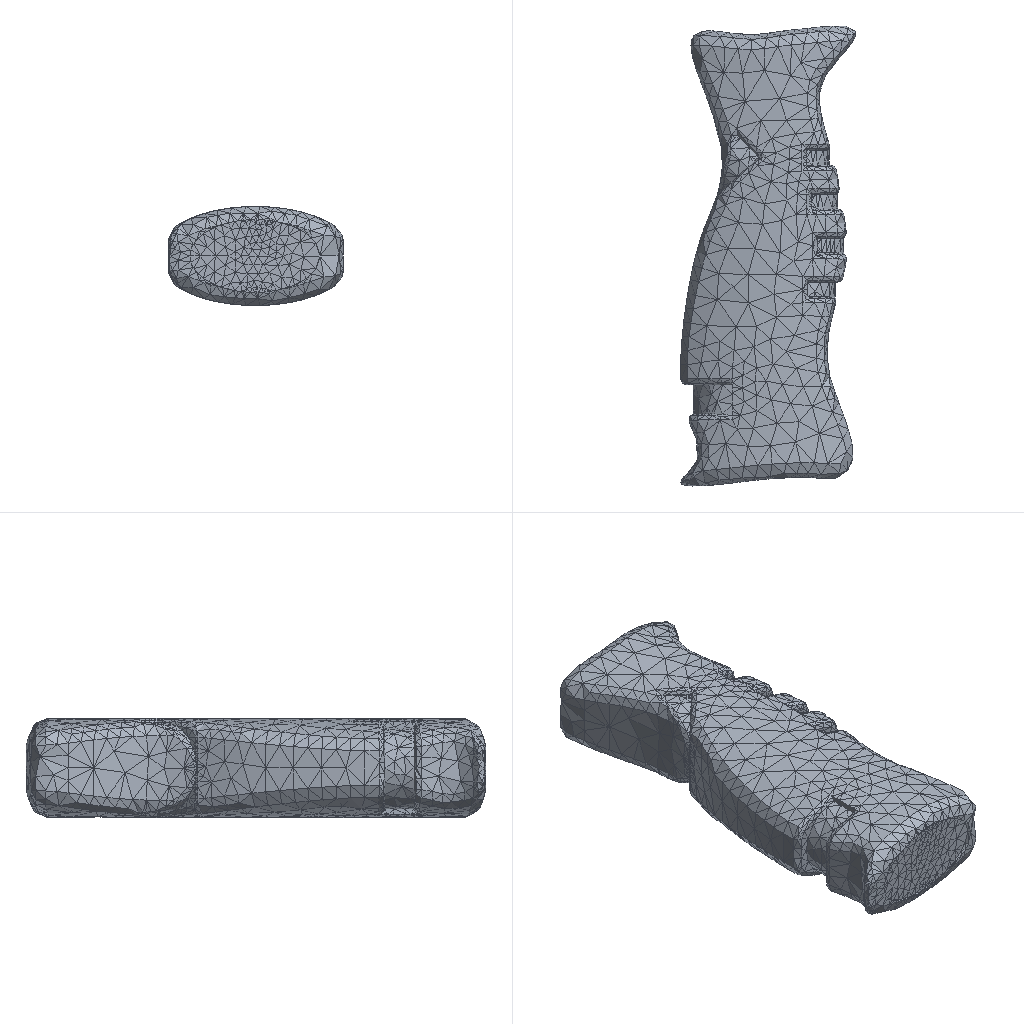Simulation study | ansys workbench
Set-up summary:
category,name,step,type,value,unit,region
solver,ansys_workbench
units,mm-N-s-tonne (MPa),,stated,"/units,MPA"
analysis,LS1,,static
load_step,LS1,LS1,static,nsubst=1; time=1
mesh,nodes,,,18022
mesh,elements,,,11020
element_type,SOLID187,,,10512
element_type,SURF154,,,508
material,Structural Steel,,E,200000,tonne s^-2 mm^-1
material,Structural Steel,,nu,0.3
material,Structural Steel,,density,7.85e-09,tonne mm^-3
material,Structural Steel,,conductivity,60.5,tonne mm s^-3 C^-1
material,Structural Steel,,specific_heat,4.34e+08,mm^2 s^-2 C^-1
material,Structural Steel,,cte,1.2e-05,C^-1
material,Structural Steel,,permeability,10000
material,Structural Steel,,resistivity,0.00017,ohm mm
load,Define Force Using Surface Effect Elements,LS1,surface-effect pres face 1,-0.8482,,SURF154 #2
bc,Fixed Supports,model,fixed,[dofs=ALL],,_FIXEDSU
named_set,_FIXEDSU,,node,961
Ansys APDL input file, long lists of numbers shortened:
/batch
/config,noeldb,1     ! force off writing results to database
*get,_wallstrt,active,,time,wall
! ANSYS input file written by Workbench version 2022 R1
! File used for geometry attach:
/title,wbnew--____ (B5)
! ****** Begin Custom Load Command Snippet ******
/COM, ACT Extensions:
/COM,     LSDYNA, 2021.1
/COM,
! ****** End   Custom Load Command Snippet ******
*DIM,_wb_ProjectScratch_dir,string,248
_wb_ProjectScratch_dir(1) = ''
*DIM,_wb_SolverFiles_dir,string,248
_wb_SolverFiles_dir(1) = ''
*DIM,_wb_userfiles_dir,string,248
_wb_userfiles_dir(1) = ''
/com,--- Data in consistent NMM units. See Solving Units in the help system for more information.
/units,MPA
/nopr
/wb,file,start              !  signify a WB generated input file
/prep7
! Turn off shape checking because checks already performed inside WB mesher.
! See help system for more information.
SHPP,OFF,,NOWARN
/nolist
etcon,set             ! allow ANSYS to choose best KEYOP's for 180x elements, resets any applicable keyopt to MAPDL defaults
/com,*********** Nodes for the whole assembly ***********
nblock,3,,19824
(1i9,3e20.9e3)
        1    -2.244507871E+01     1.630222738E+00     0.000000000E+00
! (18021 more lines like these left out)
-1
/wb,elem,start            !  set before creation of elements
/com,*********** Elements for Body 1 "Ski Grip Design Hollow22-FreeParts|Cut-Extrude9" ***********
et,1,187
eblock,19,solid,,10512
(19i9)
        1        1        1        1        0        0        0        0       10        0        1     2409     2548     2820     2619    17162    17678    17166    17163
! (21023 more lines like these left out)
-1
/wb,elem,end               !  done creating elements
/com,*********** Send User Defined Coordinate System(s) ***********
csys,0
toffst,273.15,  ! Temperature offset from absolute zero
/com,*********** Set Reference Temperature ***********
tref,22.
/wb,mat,start              !  starting to send materials
/com,*********** Send Materials ***********
Temperature = 'TEMP' ! Temperature
MP,DENS,1,7.85e-09,	! tonne mm^-3
MP,ALPX,1,1.2e-05,	! C^-1
MP,C,1,434000000,	! mm^2 s^-2 C^-1
MP,KXX,1,60.5,	! tonne mm s^-3 C^-1
MP,RSVX,1,0.00017,	! ohm mm
MP,EX,1,200000,	! tonne s^-2 mm^-1
MP,NUXY,1,0.3,
MP,MURX,1,10000,
/wb,mat,end                !  done sending materials
!************************* Model Summary ********************
!Ski Grip Design Hollow22-FreeParts|Cut-Extrude9,	结构钢,	matid,	1
!************************* End Model Summary ********************
! get the diagonal of the bounding box. Needed later for other things
*get,_xmin,node,,mnloc,x
*get,_ymin,node,,mnloc,y
*get,_zmin,node,,mnloc,z
*get,_xmax,node,,mxloc,x
*get,_ymax,node,,mxloc,y
*get,_zmax,node,,mxloc,z
_ASMDIAG=(_xmax-_xmin)*(_xmax-_xmin)+(_ymax-_ymin)*(_ymax-_ymin)+(_zmax-_zmin)*(_zmax-_zmin)
_ASMDIAG=SQRT(_ASMDIAG)
/wb,contact,start          !  starting to send contact
/wb,contact,end            !  done creating contacts
/golist
/wb,load,start             !  starting to send loads
/com,*********** Fixed Supports ***********
CMBLOCK,_FIXEDSU,NODE,      961
(8i10)
         1         2         3         4         5         6         7         8
! (120 more lines like these left out)
cmsel,s,_FIXEDSU
d,all,all
nsel,all
/com,*********** Define Force Using Surface Effect Elements ***********
local,12,0,0.,0.,0.,0.,0.,0.
csys,0
et,2,154
eblock,10,,,508
(15i9)
    14251        2        2        2       12     1646     1650     1648     1648    12750    12767     1648    12749
! (507 more lines like these left out)
-1
esel,s,type,,2
keyop,2,2,1                ! Apply load in local coordinate system
keyop,2,7,1                ! Use original area so load is constant in large deformation
esel,all
/gst,on,on
fini
*get,_numnode,node,0,count
*get,_numelem,elem,0,count
*get, _MAXELEMNUM, elem, 0, NUM, MAX
*get, _MAXNODENUM, node, 0, NUM, MAX
*get, _MAXELEMTYPE, etyp, 0, NUM, MAX
*get, _MAXREALCONST, real, 0, NUM, MAX
/go
/wb,load,end               !  done creating loads
/com,--- Number of total nodes = %_numnode%
/com,--- Number of contact elements = 508
/com,--- Number of spring elements = 0
/com,--- Number of bearing elements = 0
/com,--- Number of solid elements = 10512
/com,--- Number of condensed parts = 0
/com,--- Number of total elements = %_numelem%
*get,_wallbsol,active,,time,wall
/com,****************************************************************************
/com,*************************    SOLUTION       ********************************
/com,****************************************************************************
/solu
antype,0                   ! static analysis
_thickRatio=  1     ! Ratio of thick parts in the model
eqsl,pcg,1e-8,,,,,,1
cntr,print,1               ! print out contact info and also make no initial contact an error
dmpoption,emat,no             ! Don't combine emat file for DANSYS
dmpoption,esav,no             ! Don't combine esav file for DANSYS
nldiag,cont,iter           ! print out contact info each equilibrium iteration
rescontrol,,none                 ! Do not keep any restart files
/com,****************************************************
/com,******************* SOLVE FOR LS 1 OF 1 ****************
esel,s,type,,2
nsle
sfe,all,1,pres,1,-0.8482
sfe,all,2,pres,1,0.
sfe,all,3,pres,1,0.
nsel,all
esel,all
/nopr
/gopr
nsub,1,1,1
time,1.
outres,erase
outres,all,none
outres,nsol,all,
outres,rsol,all
outres,eangl,all
outres,etmp,all
outres,veng,all
outres,strs,all,
outres,epel,all,
outres,eppl,all,
outres,cont,all,
! *********** WB SOLVE COMMAND ***********
! check interactive state
*get,ANSINTER_,active,,int
*if,ANSINTER_,ne,0,then
/eof
*endif
solve
/com *************** Write FE CONNECTORS *********
CEWRITE,file,ce,,INTE
/com,****************************************************
/com,*************** FINISHED SOLVE FOR LS 1 *************
*get,_wallasol,active,,time,wall
/nopr
*get,_numnode,node,0,count
*get,_numelem,elem,0,count
*get, _MAXELEMNUM, elem, 0, NUM, MAX
*get, _MAXNODENUM, node, 0, NUM, MAX,,,INTERNAL
*get, _MAXELEMTYPE, etyp, 0, NUM, MAX
*get, _MAXREALCONST, real, 0, NUM, MAX
/gopr
*get,_PCGITER,active,,solu,cgiter
/post1
xmlo,ENCODING,ISO-8859-1
xmlo,parm
/xml,parm,xml
fini
/gopr
*get,_walldone,active,,time,wall
_preptime=(_wallbsol-_wallstrt)*3600
_solvtime=(_wallasol-_wallbsol)*3600
_posttime=(_walldone-_wallasol)*3600
_totaltim=(_walldone-_wallstrt)*3600
*get,_dlbratio,active,0,solu,dlbr
*get,_combtime,active,0,solu,comb
*get,_ssmode,active,0,solu,ssmm
*get,_ndofs,active,0,solu,ndof
*get,_sol_end_time,active,0,set,time
*if,_sol_end_time,eq,1.,then
/fclean				!clean distributed files
*endif
/com,--- Total number of nodes = %_numnode%
/com,--- Total number of elements = %_numelem%
/com,--- Element load balance ratio = %_dlbratio%
/com,--- Time to combine distributed files = %_combtime%
/com,--- Sparse memory mode = %_ssmode%
/com,--- Number of DOF = %_ndofs%
/wb,file,end               ! done with WB generated input
Results summary:
result,analyses[0].index,,,1
result,analyses[0].system,,,SYS
result,analyses[0].deck,,,deck.dat
result,analyses[0].solve_status,,,completed
result,analyses[0].analysis_type,,,static
result,analyses[0].physics,,,mechanical
result,analyses[0].unit_system,,,"NMM: mm, ton, N, s, mV, mA, degC"
result,analyses[0].n_sets,,,1
result,analyses[0].load_steps[0].set,set=1,,1
result,analyses[0].load_steps[0].time_or_freq,set=1,,1
result,analyses[0].load_steps[0].max_displacement_magnitude,set=1,,0.0006317
result,analyses[0].load_steps[0].max_von_mises_nodal,set=1,,20.812
result,analyses[0].load_steps[0].reaction_force_sum_xyz[1],set=1,,4999.93
result,analyses[0].load_steps[0].reaction_force_sum_xyz[2],set=1,,1.52309e-06
result,analyses[0].load_steps[0].reaction_force_sum_xyz[3],set=1,,-3.49005e-07